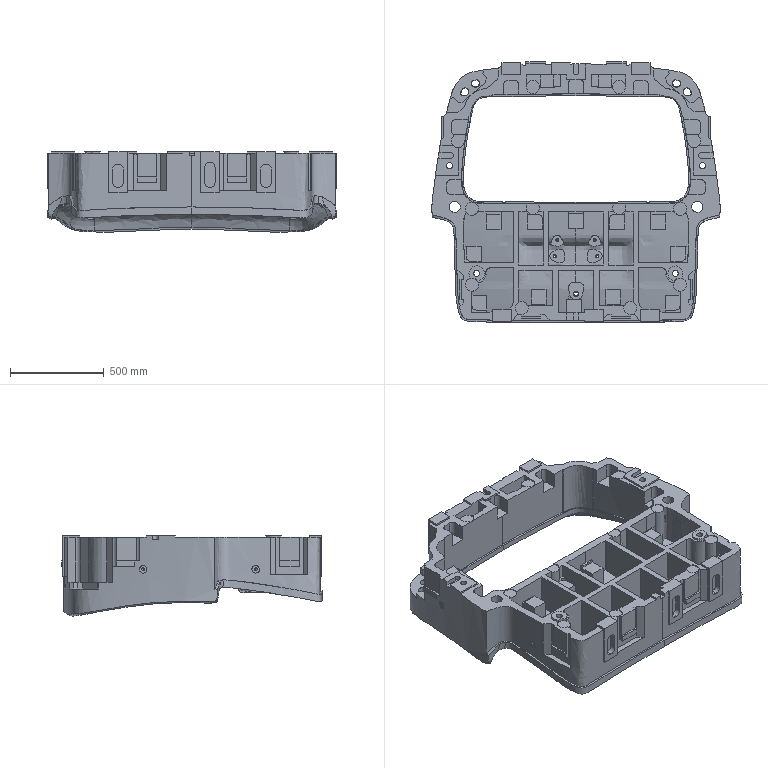Part | NX | features solid 2 | 1 solid | 917 faces | box 1540 x 1390 x 431.213 mm | volume 202741510 mm3 | plane 448 | spline 313 | cylinder 150 | cone 6 | commonest cylinder face diameters 50 x28 70 x23 44 x20 60 x11 16 x9 40 x7